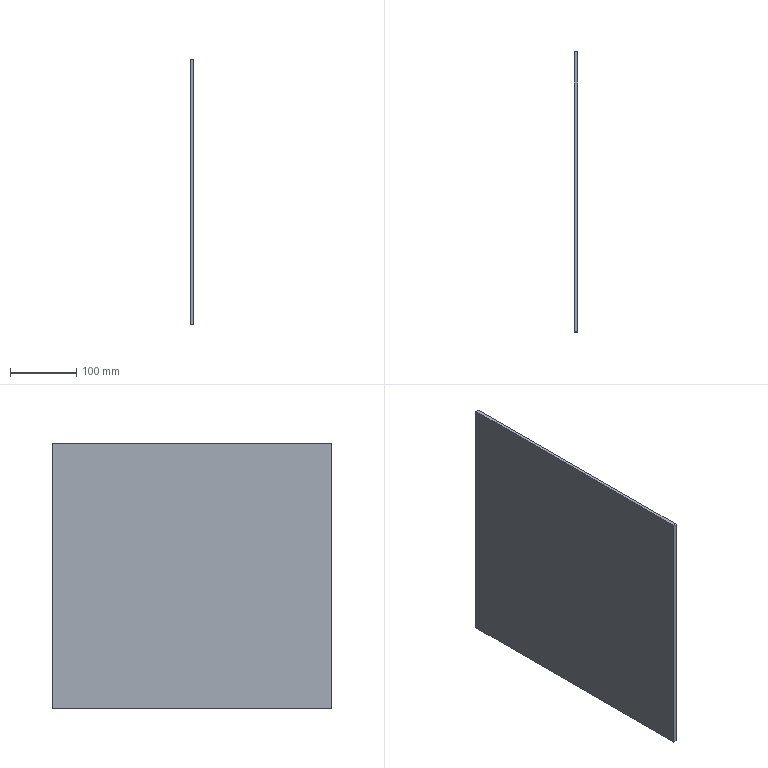Part | STEP file | Guide wheel mechanism revised.sldasm-Part-183 | 1 solid | 6 faces | box 5 x 421.99 x 400 mm | volume 843980 mm3 | plane 6
STEP:
#1=CARTESIAN_POINT('',(440.,1910.,200.));
#2=VERTEX_POINT('',#1);
#3=CARTESIAN_POINT('',(440.,1488.01,200.));
#4=VERTEX_POINT('',#3);
#5=CARTESIAN_POINT('',(440.,1910.,200.));
#6=DIRECTION('',(0.,-1.,0.));
#7=VECTOR('',#6,1000.);
#8=LINE('',#5,#7);
#9=EDGE_CURVE('',#2,#4,#8,.T.);
#10=ORIENTED_EDGE('',*,*,#9,.F.);
#11=CARTESIAN_POINT('',(435.,1910.,200.));
#12=VERTEX_POINT('',#11);
#13=CARTESIAN_POINT('',(435.,1910.,200.));
#14=DIRECTION('',(1.,0.,0.));
#15=VECTOR('',#14,1000.);
#16=LINE('',#13,#15);
#17=EDGE_CURVE('',#12,#2,#16,.T.);
#18=ORIENTED_EDGE('',*,*,#17,.F.);
#19=CARTESIAN_POINT('',(435.,1488.01,200.));
#20=VERTEX_POINT('',#19);
#21=CARTESIAN_POINT('',(435.,1910.,200.));
#22=DIRECTION('',(0.,-1.,0.));
#23=VECTOR('',#22,1000.);
#24=LINE('',#21,#23);
#25=EDGE_CURVE('',#12,#20,#24,.T.);
#26=ORIENTED_EDGE('',*,*,#25,.T.);
#27=CARTESIAN_POINT('',(435.,1488.01,200.));
#28=DIRECTION('',(1.,0.,0.));
#29=VECTOR('',#28,1000.);
#30=LINE('',#27,#29);
#31=EDGE_CURVE('',#20,#4,#30,.T.);
#32=ORIENTED_EDGE('',*,*,#31,.T.);
#33=EDGE_LOOP('',(#10,#18,#26,#32));
#34=FACE_OUTER_BOUND('',#33,.T.);
#35=CARTESIAN_POINT('',(435.,1910.,200.));
#36=DIRECTION('',(0.,0.,1.));
#37=DIRECTION('',(0.,-1.,0.));
#38=AXIS2_PLACEMENT_3D('',#35,#36,#37);
#39=PLANE('',#38);
#40=ADVANCED_FACE('',(#34),#39,.T.);
#41=CARTESIAN_POINT('',(440.,1910.,-200.));
#42=VERTEX_POINT('',#41);
#43=CARTESIAN_POINT('',(440.,1910.,200.));
#44=DIRECTION('',(0.,0.,1.));
#45=VECTOR('',#44,1000.);
#46=LINE('',#43,#45);
#47=EDGE_CURVE('',#42,#2,#46,.T.);
#48=ORIENTED_EDGE('',*,*,#47,.F.);
#49=CARTESIAN_POINT('',(435.,1910.,-200.));
#50=VERTEX_POINT('',#49);
#51=CARTESIAN_POINT('',(435.,1910.,-200.));
#52=DIRECTION('',(1.,0.,0.));
#53=VECTOR('',#52,1000.);
#54=LINE('',#51,#53);
#55=EDGE_CURVE('',#50,#42,#54,.T.);
#56=ORIENTED_EDGE('',*,*,#55,.F.);
#57=CARTESIAN_POINT('',(435.,1910.,200.));
#58=DIRECTION('',(0.,0.,1.));
#59=VECTOR('',#58,1000.);
#60=LINE('',#57,#59);
#61=EDGE_CURVE('',#50,#12,#60,.T.);
#62=ORIENTED_EDGE('',*,*,#61,.T.);
#63=ORIENTED_EDGE('',*,*,#17,.T.);
#64=EDGE_LOOP('',(#48,#56,#62,#63));
#65=FACE_OUTER_BOUND('',#64,.T.);
#66=CARTESIAN_POINT('',(435.,1910.,200.));
#67=DIRECTION('',(0.,1.,0.));
#68=DIRECTION('',(0.,0.,1.));
#69=AXIS2_PLACEMENT_3D('',#66,#67,#68);
#70=PLANE('',#69);
#71=ADVANCED_FACE('',(#65),#70,.T.);
#72=CARTESIAN_POINT('',(440.,1488.01,-200.));
#73=VERTEX_POINT('',#72);
#74=CARTESIAN_POINT('',(440.,1910.,-200.));
#75=DIRECTION('',(0.,1.,0.));
#76=VECTOR('',#75,1000.);
#77=LINE('',#74,#76);
#78=EDGE_CURVE('',#73,#42,#77,.T.);
#79=ORIENTED_EDGE('',*,*,#78,.F.);
#80=CARTESIAN_POINT('',(435.,1488.01,-200.));
#81=VERTEX_POINT('',#80);
#82=CARTESIAN_POINT('',(435.,1488.01,-200.));
#83=DIRECTION('',(1.,0.,0.));
#84=VECTOR('',#83,1000.);
#85=LINE('',#82,#84);
#86=EDGE_CURVE('',#81,#73,#85,.T.);
#87=ORIENTED_EDGE('',*,*,#86,.F.);
#88=CARTESIAN_POINT('',(435.,1910.,-200.));
#89=DIRECTION('',(0.,1.,0.));
#90=VECTOR('',#89,1000.);
#91=LINE('',#88,#90);
#92=EDGE_CURVE('',#81,#50,#91,.T.);
#93=ORIENTED_EDGE('',*,*,#92,.T.);
#94=ORIENTED_EDGE('',*,*,#55,.T.);
#95=EDGE_LOOP('',(#79,#87,#93,#94));
#96=FACE_OUTER_BOUND('',#95,.T.);
#97=CARTESIAN_POINT('',(435.,1910.,-200.));
#98=DIRECTION('',(0.,0.,-1.));
#99=DIRECTION('',(0.,1.,0.));
#100=AXIS2_PLACEMENT_3D('',#97,#98,#99);
#101=PLANE('',#100);
#102=ADVANCED_FACE('',(#96),#101,.T.);
#103=CARTESIAN_POINT('',(440.,1488.01,200.));
#104=DIRECTION('',(0.,0.,-1.));
#105=VECTOR('',#104,1000.);
#106=LINE('',#103,#105);
#107=EDGE_CURVE('',#4,#73,#106,.T.);
#108=ORIENTED_EDGE('',*,*,#107,.F.);
#109=ORIENTED_EDGE('',*,*,#31,.F.);
#110=CARTESIAN_POINT('',(435.,1488.01,200.));
#111=DIRECTION('',(0.,0.,-1.));
#112=VECTOR('',#111,1000.);
#113=LINE('',#110,#112);
#114=EDGE_CURVE('',#20,#81,#113,.T.);
#115=ORIENTED_EDGE('',*,*,#114,.T.);
#116=ORIENTED_EDGE('',*,*,#86,.T.);
#117=EDGE_LOOP('',(#108,#109,#115,#116));
#118=FACE_OUTER_BOUND('',#117,.T.);
#119=CARTESIAN_POINT('',(435.,1488.01,200.));
#120=DIRECTION('',(0.,-1.,0.));
#121=DIRECTION('',(0.,0.,-1.));
#122=AXIS2_PLACEMENT_3D('',#119,#120,#121);
#123=PLANE('',#122);
#124=ADVANCED_FACE('',(#118),#123,.T.);
#125=ORIENTED_EDGE('',*,*,#25,.F.);
#126=ORIENTED_EDGE('',*,*,#61,.F.);
#127=ORIENTED_EDGE('',*,*,#92,.F.);
#128=ORIENTED_EDGE('',*,*,#114,.F.);
#129=EDGE_LOOP('',(#125,#126,#127,#128));
#130=FACE_OUTER_BOUND('',#129,.T.);
#131=CARTESIAN_POINT('',(435.,0.,0.));
#132=DIRECTION('',(1.,0.,0.));
#133=DIRECTION('',(0.,0.,-1.));
#134=AXIS2_PLACEMENT_3D('',#131,#132,#133);
#135=PLANE('',#134);
#136=ADVANCED_FACE('',(#130),#135,.F.);
#137=ORIENTED_EDGE('',*,*,#9,.T.);
#138=ORIENTED_EDGE('',*,*,#107,.T.);
#139=ORIENTED_EDGE('',*,*,#78,.T.);
#140=ORIENTED_EDGE('',*,*,#47,.T.);
#141=EDGE_LOOP('',(#137,#138,#139,#140));
#142=FACE_OUTER_BOUND('',#141,.T.);
#143=CARTESIAN_POINT('',(440.,0.,0.));
#144=DIRECTION('',(1.,0.,0.));
#145=DIRECTION('',(0.,0.,-1.));
#146=AXIS2_PLACEMENT_3D('',#143,#144,#145);
#147=PLANE('',#146);
#148=ADVANCED_FACE('',(#142),#147,.T.);
#149=CLOSED_SHELL('',(#40,#71,#102,#124,#136,#148));
#150=MANIFOLD_SOLID_BREP('',#149);
#151=CARTESIAN_POINT('',(0.,0.,0.));
#152=DIRECTION('',(0.,0.,1.));
#153=DIRECTION('',(1.,0.,0.));
#154=AXIS2_PLACEMENT_3D('',#151,#152,#153);
#155=(LENGTH_UNIT()NAMED_UNIT(*)SI_UNIT(.MILLI.,.METRE.));
#156=UNCERTAINTY_MEASURE_WITH_UNIT(LENGTH_MEASURE(0.00001),#155,'','');
#157=(NAMED_UNIT(*)PLANE_ANGLE_UNIT()SI_UNIT($,.RADIAN.));
#158=(NAMED_UNIT(*)SI_UNIT($,.STERADIAN.)SOLID_ANGLE_UNIT());
#159=(GEOMETRIC_REPRESENTATION_CONTEXT(3)GLOBAL_UNCERTAINTY_ASSIGNED_CONTEXT((#156))GLOBAL_UNIT_ASSIGNED_CONTEXT((#155,#157,#158))REPRESENTATION_CONTEXT('',''));
#160=ADVANCED_BREP_SHAPE_REPRESENTATION('',(#150,#154),#159);